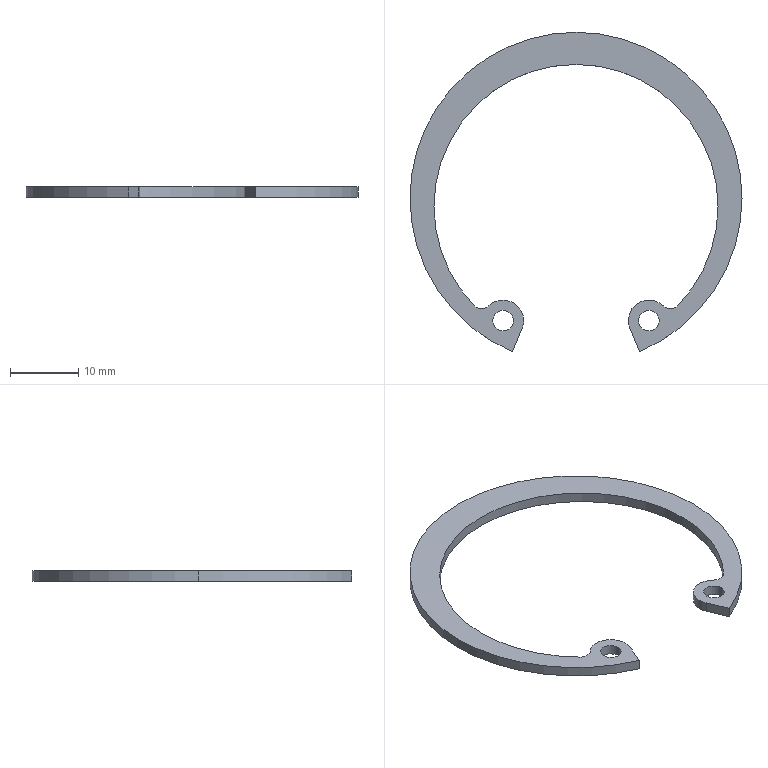Part | STEP file | circlips for holes--type a gb_GB_CONNECTING_PIECE_RING_RRH 45 | 1 solid | 19 faces | box 48.5 x 46.654 x 1.5 mm | volume 718.222 mm3 | cylinder 15 | plane 4 | commonest cylinder face diameters 3 x6 6 x3 41.5 x3 48.5 x3
STEP:
#1=CARTESIAN_POINT('',(24.25,0.,-1.5));
#2=VERTEX_POINT('',#1);
#3=CARTESIAN_POINT('',(-24.25,0.,-1.5));
#4=VERTEX_POINT('',#3);
#5=CARTESIAN_POINT('',(0.,0.,-1.5));
#6=DIRECTION('',(0.,0.,1.));
#7=DIRECTION('',(1.,0.,0.));
#8=AXIS2_PLACEMENT_3D('',#5,#6,#7);
#9=CIRCLE('',#8,24.25);
#10=EDGE_CURVE('',#2,#4,#9,.T.);
#11=ORIENTED_EDGE('',*,*,#10,.T.);
#12=CARTESIAN_POINT('',(-24.25,0.,0.));
#13=VERTEX_POINT('',#12);
#14=CARTESIAN_POINT('',(-24.25,0.,-1.5));
#15=DIRECTION('',(0.,0.,1.));
#16=VECTOR('',#15,1000.);
#17=LINE('',#14,#16);
#18=EDGE_CURVE('',#4,#13,#17,.T.);
#19=ORIENTED_EDGE('',*,*,#18,.T.);
#20=CARTESIAN_POINT('',(24.25,0.,0.));
#21=VERTEX_POINT('',#20);
#22=CARTESIAN_POINT('',(0.,0.,0.));
#23=DIRECTION('',(0.,0.,-1.));
#24=DIRECTION('',(1.,0.,0.));
#25=AXIS2_PLACEMENT_3D('',#22,#23,#24);
#26=CIRCLE('',#25,24.25);
#27=EDGE_CURVE('',#13,#21,#26,.T.);
#28=ORIENTED_EDGE('',*,*,#27,.T.);
#29=CARTESIAN_POINT('',(24.25,0.,-1.5));
#30=DIRECTION('',(0.,0.,1.));
#31=VECTOR('',#30,1000.);
#32=LINE('',#29,#31);
#33=EDGE_CURVE('',#2,#21,#32,.T.);
#34=ORIENTED_EDGE('',*,*,#33,.F.);
#35=EDGE_LOOP('',(#11,#19,#28,#34));
#36=FACE_OUTER_BOUND('',#35,.T.);
#37=CARTESIAN_POINT('',(0.,0.,-1.5));
#38=DIRECTION('',(0.,0.,1.));
#39=DIRECTION('',(1.,0.,0.));
#40=AXIS2_PLACEMENT_3D('',#37,#38,#39);
#41=CYLINDRICAL_SURFACE('',#40,24.25);
#42=ADVANCED_FACE('',(#36),#41,.T.);
#43=CARTESIAN_POINT('',(9.28,-22.404,-1.5));
#44=VERTEX_POINT('',#43);
#45=CARTESIAN_POINT('',(0.,0.,-1.5));
#46=DIRECTION('',(0.,0.,1.));
#47=DIRECTION('',(1.,0.,0.));
#48=AXIS2_PLACEMENT_3D('',#45,#46,#47);
#49=CIRCLE('',#48,24.25);
#50=EDGE_CURVE('',#44,#2,#49,.T.);
#51=ORIENTED_EDGE('',*,*,#50,.T.);
#52=ORIENTED_EDGE('',*,*,#33,.T.);
#53=CARTESIAN_POINT('',(9.28,-22.404,0.));
#54=VERTEX_POINT('',#53);
#55=CARTESIAN_POINT('',(0.,0.,0.));
#56=DIRECTION('',(0.,0.,-1.));
#57=DIRECTION('',(1.,0.,0.));
#58=AXIS2_PLACEMENT_3D('',#55,#56,#57);
#59=CIRCLE('',#58,24.25);
#60=EDGE_CURVE('',#21,#54,#59,.T.);
#61=ORIENTED_EDGE('',*,*,#60,.T.);
#62=CARTESIAN_POINT('',(9.28,-22.404,-1.5));
#63=DIRECTION('',(0.,0.,-1.));
#64=VECTOR('',#63,1000.);
#65=LINE('',#62,#64);
#66=EDGE_CURVE('',#54,#44,#65,.T.);
#67=ORIENTED_EDGE('',*,*,#66,.T.);
#68=EDGE_LOOP('',(#51,#52,#61,#67));
#69=FACE_OUTER_BOUND('',#68,.T.);
#70=CARTESIAN_POINT('',(0.,0.,-1.5));
#71=DIRECTION('',(0.,0.,1.));
#72=DIRECTION('',(1.,0.,0.));
#73=AXIS2_PLACEMENT_3D('',#70,#71,#72);
#74=CYLINDRICAL_SURFACE('',#73,24.25);
#75=ADVANCED_FACE('',(#69),#74,.T.);
#76=CARTESIAN_POINT('',(-14.857,-15.686,-1.5));
#77=VERTEX_POINT('',#76);
#78=CARTESIAN_POINT('',(-20.75,-1.2,-1.5));
#79=VERTEX_POINT('',#78);
#80=CARTESIAN_POINT('',(0.,-1.2,-1.5));
#81=DIRECTION('',(0.,0.,-1.));
#82=DIRECTION('',(1.,0.,0.));
#83=AXIS2_PLACEMENT_3D('',#80,#81,#82);
#84=CIRCLE('',#83,20.75);
#85=EDGE_CURVE('',#77,#79,#84,.T.);
#86=ORIENTED_EDGE('',*,*,#85,.T.);
#87=CARTESIAN_POINT('',(-20.75,-1.2,0.));
#88=VERTEX_POINT('',#87);
#89=CARTESIAN_POINT('',(-20.75,-1.2,-1.5));
#90=DIRECTION('',(0.,0.,1.));
#91=VECTOR('',#90,1000.);
#92=LINE('',#89,#91);
#93=EDGE_CURVE('',#79,#88,#92,.T.);
#94=ORIENTED_EDGE('',*,*,#93,.T.);
#95=CARTESIAN_POINT('',(-14.857,-15.686,0.));
#96=VERTEX_POINT('',#95);
#97=CARTESIAN_POINT('',(0.,-1.2,0.));
#98=DIRECTION('',(0.,0.,-1.));
#99=DIRECTION('',(1.,0.,0.));
#100=AXIS2_PLACEMENT_3D('',#97,#98,#99);
#101=CIRCLE('',#100,20.75);
#102=EDGE_CURVE('',#96,#88,#101,.T.);
#103=ORIENTED_EDGE('',*,*,#102,.F.);
#104=CARTESIAN_POINT('',(-14.857,-15.686,-1.5));
#105=DIRECTION('',(0.,0.,1.));
#106=VECTOR('',#105,1000.);
#107=LINE('',#104,#106);
#108=EDGE_CURVE('',#77,#96,#107,.T.);
#109=ORIENTED_EDGE('',*,*,#108,.F.);
#110=EDGE_LOOP('',(#86,#94,#103,#109));
#111=FACE_OUTER_BOUND('',#110,.T.);
#112=CARTESIAN_POINT('',(0.,-1.2,-1.5));
#113=DIRECTION('',(0.,0.,1.));
#114=DIRECTION('',(1.,0.,0.));
#115=AXIS2_PLACEMENT_3D('',#112,#113,#114);
#116=CYLINDRICAL_SURFACE('',#115,20.75);
#117=ADVANCED_FACE('',(#111),#116,.F.);
#118=ORIENTED_EDGE('',*,*,#93,.F.);
#119=CARTESIAN_POINT('',(20.75,-1.2,-1.5));
#120=VERTEX_POINT('',#119);
#121=CARTESIAN_POINT('',(0.,-1.2,-1.5));
#122=DIRECTION('',(0.,0.,-1.));
#123=DIRECTION('',(1.,0.,0.));
#124=AXIS2_PLACEMENT_3D('',#121,#122,#123);
#125=CIRCLE('',#124,20.75);
#126=EDGE_CURVE('',#79,#120,#125,.T.);
#127=ORIENTED_EDGE('',*,*,#126,.T.);
#128=CARTESIAN_POINT('',(20.75,-1.2,0.));
#129=VERTEX_POINT('',#128);
#130=CARTESIAN_POINT('',(20.75,-1.2,-1.5));
#131=DIRECTION('',(0.,0.,1.));
#132=VECTOR('',#131,1000.);
#133=LINE('',#130,#132);
#134=EDGE_CURVE('',#120,#129,#133,.T.);
#135=ORIENTED_EDGE('',*,*,#134,.T.);
#136=CARTESIAN_POINT('',(0.,-1.2,0.));
#137=DIRECTION('',(0.,0.,-1.));
#138=DIRECTION('',(1.,0.,0.));
#139=AXIS2_PLACEMENT_3D('',#136,#137,#138);
#140=CIRCLE('',#139,20.75);
#141=EDGE_CURVE('',#88,#129,#140,.T.);
#142=ORIENTED_EDGE('',*,*,#141,.F.);
#143=EDGE_LOOP('',(#118,#127,#135,#142));
#144=FACE_OUTER_BOUND('',#143,.T.);
#145=CARTESIAN_POINT('',(0.,-1.2,-1.5));
#146=DIRECTION('',(0.,0.,1.));
#147=DIRECTION('',(1.,0.,0.));
#148=AXIS2_PLACEMENT_3D('',#145,#146,#147);
#149=CYLINDRICAL_SURFACE('',#148,20.75);
#150=ADVANCED_FACE('',(#144),#149,.F.);
#151=CARTESIAN_POINT('',(-7.877,-19.016,-1.5));
#152=VERTEX_POINT('',#151);
#153=CARTESIAN_POINT('',(-7.648,-17.868,-1.5));
#154=VERTEX_POINT('',#153);
#155=CARTESIAN_POINT('',(-10.648,-17.868,-1.5));
#156=DIRECTION('',(0.,0.,1.));
#157=DIRECTION('',(1.,0.,0.));
#158=AXIS2_PLACEMENT_3D('',#155,#156,#157);
#159=CIRCLE('',#158,3.);
#160=EDGE_CURVE('',#152,#154,#159,.T.);
#161=ORIENTED_EDGE('',*,*,#160,.T.);
#162=CARTESIAN_POINT('',(-7.648,-17.868,0.));
#163=VERTEX_POINT('',#162);
#164=CARTESIAN_POINT('',(-7.648,-17.868,-1.5));
#165=DIRECTION('',(0.,0.,1.));
#166=VECTOR('',#165,1000.);
#167=LINE('',#164,#166);
#168=EDGE_CURVE('',#154,#163,#167,.T.);
#169=ORIENTED_EDGE('',*,*,#168,.T.);
#170=CARTESIAN_POINT('',(-7.877,-19.016,0.));
#171=VERTEX_POINT('',#170);
#172=CARTESIAN_POINT('',(-10.648,-17.868,0.));
#173=DIRECTION('',(0.,0.,-1.));
#174=DIRECTION('',(1.,0.,0.));
#175=AXIS2_PLACEMENT_3D('',#172,#173,#174);
#176=CIRCLE('',#175,3.);
#177=EDGE_CURVE('',#163,#171,#176,.T.);
#178=ORIENTED_EDGE('',*,*,#177,.T.);
#179=CARTESIAN_POINT('',(-7.877,-19.016,-1.5));
#180=DIRECTION('',(0.,0.,-1.));
#181=VECTOR('',#180,1000.);
#182=LINE('',#179,#181);
#183=EDGE_CURVE('',#171,#152,#182,.T.);
#184=ORIENTED_EDGE('',*,*,#183,.T.);
#185=EDGE_LOOP('',(#161,#169,#178,#184));
#186=FACE_OUTER_BOUND('',#185,.T.);
#187=CARTESIAN_POINT('',(-10.648,-17.868,-1.5));
#188=DIRECTION('',(0.,0.,1.));
#189=DIRECTION('',(1.,0.,0.));
#190=AXIS2_PLACEMENT_3D('',#187,#188,#189);
#191=CYLINDRICAL_SURFACE('',#190,3.);
#192=ADVANCED_FACE('',(#186),#191,.T.);
#193=CARTESIAN_POINT('',(12.148,-17.868,-1.5));
#194=VERTEX_POINT('',#193);
#195=CARTESIAN_POINT('',(9.148,-17.868,-1.5));
#196=VERTEX_POINT('',#195);
#197=CARTESIAN_POINT('',(10.648,-17.868,-1.5));
#198=DIRECTION('',(0.,0.,-1.));
#199=DIRECTION('',(1.,0.,0.));
#200=AXIS2_PLACEMENT_3D('',#197,#198,#199);
#201=CIRCLE('',#200,1.5);
#202=EDGE_CURVE('',#194,#196,#201,.T.);
#203=ORIENTED_EDGE('',*,*,#202,.T.);
#204=CARTESIAN_POINT('',(9.148,-17.868,0.));
#205=VERTEX_POINT('',#204);
#206=CARTESIAN_POINT('',(9.148,-17.868,-1.5));
#207=DIRECTION('',(0.,0.,1.));
#208=VECTOR('',#207,1000.);
#209=LINE('',#206,#208);
#210=EDGE_CURVE('',#196,#205,#209,.T.);
#211=ORIENTED_EDGE('',*,*,#210,.T.);
#212=CARTESIAN_POINT('',(12.148,-17.868,0.));
#213=VERTEX_POINT('',#212);
#214=CARTESIAN_POINT('',(10.648,-17.868,0.));
#215=DIRECTION('',(0.,0.,-1.));
#216=DIRECTION('',(1.,0.,0.));
#217=AXIS2_PLACEMENT_3D('',#214,#215,#216);
#218=CIRCLE('',#217,1.5);
#219=EDGE_CURVE('',#213,#205,#218,.T.);
#220=ORIENTED_EDGE('',*,*,#219,.F.);
#221=CARTESIAN_POINT('',(12.148,-17.868,-1.5));
#222=DIRECTION('',(0.,0.,1.));
#223=VECTOR('',#222,1000.);
#224=LINE('',#221,#223);
#225=EDGE_CURVE('',#194,#213,#224,.T.);
#226=ORIENTED_EDGE('',*,*,#225,.F.);
#227=EDGE_LOOP('',(#203,#211,#220,#226));
#228=FACE_OUTER_BOUND('',#227,.T.);
#229=CARTESIAN_POINT('',(10.648,-17.868,-1.5));
#230=DIRECTION('',(0.,0.,1.));
#231=DIRECTION('',(1.,0.,0.));
#232=AXIS2_PLACEMENT_3D('',#229,#230,#231);
#233=CYLINDRICAL_SURFACE('',#232,1.5);
#234=ADVANCED_FACE('',(#228),#233,.F.);
#235=CARTESIAN_POINT('',(-9.148,-17.868,-1.5));
#236=VERTEX_POINT('',#235);
#237=CARTESIAN_POINT('',(-12.148,-17.868,-1.5));
#238=VERTEX_POINT('',#237);
#239=CARTESIAN_POINT('',(-10.648,-17.868,-1.5));
#240=DIRECTION('',(0.,0.,-1.));
#241=DIRECTION('',(1.,0.,0.));
#242=AXIS2_PLACEMENT_3D('',#239,#240,#241);
#243=CIRCLE('',#242,1.5);
#244=EDGE_CURVE('',#236,#238,#243,.T.);
#245=ORIENTED_EDGE('',*,*,#244,.T.);
#246=CARTESIAN_POINT('',(-12.148,-17.868,0.));
#247=VERTEX_POINT('',#246);
#248=CARTESIAN_POINT('',(-12.148,-17.868,-1.5));
#249=DIRECTION('',(0.,0.,1.));
#250=VECTOR('',#249,1000.);
#251=LINE('',#248,#250);
#252=EDGE_CURVE('',#238,#247,#251,.T.);
#253=ORIENTED_EDGE('',*,*,#252,.T.);
#254=CARTESIAN_POINT('',(-9.148,-17.868,0.));
#255=VERTEX_POINT('',#254);
#256=CARTESIAN_POINT('',(-10.648,-17.868,0.));
#257=DIRECTION('',(0.,0.,-1.));
#258=DIRECTION('',(1.,0.,0.));
#259=AXIS2_PLACEMENT_3D('',#256,#257,#258);
#260=CIRCLE('',#259,1.5);
#261=EDGE_CURVE('',#255,#247,#260,.T.);
#262=ORIENTED_EDGE('',*,*,#261,.F.);
#263=CARTESIAN_POINT('',(-9.148,-17.868,-1.5));
#264=DIRECTION('',(0.,0.,1.));
#265=VECTOR('',#264,1000.);
#266=LINE('',#263,#265);
#267=EDGE_CURVE('',#236,#255,#266,.T.);
#268=ORIENTED_EDGE('',*,*,#267,.F.);
#269=EDGE_LOOP('',(#245,#253,#262,#268));
#270=FACE_OUTER_BOUND('',#269,.T.);
#271=CARTESIAN_POINT('',(-10.648,-17.868,-1.5));
#272=DIRECTION('',(0.,0.,1.));
#273=DIRECTION('',(1.,0.,0.));
#274=AXIS2_PLACEMENT_3D('',#271,#272,#273);
#275=CYLINDRICAL_SURFACE('',#274,1.5);
#276=ADVANCED_FACE('',(#270),#275,.F.);
#277=CARTESIAN_POINT('',(7.877,-19.016,-1.5));
#278=VERTEX_POINT('',#277);
#279=CARTESIAN_POINT('',(7.877,-19.016,-1.5));
#280=DIRECTION('',(0.3827,-0.9239,0.));
#281=VECTOR('',#280,1000.);
#282=LINE('',#279,#281);
#283=EDGE_CURVE('',#278,#44,#282,.T.);
#284=ORIENTED_EDGE('',*,*,#283,.F.);
#285=CARTESIAN_POINT('',(12.738,-15.715,-1.5));
#286=VERTEX_POINT('',#285);
#287=CARTESIAN_POINT('',(10.648,-17.868,-1.5));
#288=DIRECTION('',(0.,0.,1.));
#289=DIRECTION('',(1.,0.,0.));
#290=AXIS2_PLACEMENT_3D('',#287,#288,#289);
#291=CIRCLE('',#290,3.);
#292=EDGE_CURVE('',#286,#278,#291,.T.);
#293=ORIENTED_EDGE('',*,*,#292,.F.);
#294=CARTESIAN_POINT('',(14.857,-15.686,-1.5));
#295=VERTEX_POINT('',#294);
#296=CARTESIAN_POINT('',(13.783,-14.639,-1.5));
#297=DIRECTION('',(0.,0.,-1.));
#298=DIRECTION('',(1.,0.,0.));
#299=AXIS2_PLACEMENT_3D('',#296,#297,#298);
#300=CIRCLE('',#299,1.5);
#301=EDGE_CURVE('',#295,#286,#300,.T.);
#302=ORIENTED_EDGE('',*,*,#301,.F.);
#303=CARTESIAN_POINT('',(0.,-1.2,-1.5));
#304=DIRECTION('',(0.,0.,-1.));
#305=DIRECTION('',(1.,0.,0.));
#306=AXIS2_PLACEMENT_3D('',#303,#304,#305);
#307=CIRCLE('',#306,20.75);
#308=EDGE_CURVE('',#120,#295,#307,.T.);
#309=ORIENTED_EDGE('',*,*,#308,.F.);
#310=ORIENTED_EDGE('',*,*,#126,.F.);
#311=ORIENTED_EDGE('',*,*,#85,.F.);
#312=CARTESIAN_POINT('',(-12.738,-15.715,-1.5));
#313=VERTEX_POINT('',#312);
#314=CARTESIAN_POINT('',(-13.783,-14.639,-1.5));
#315=DIRECTION('',(0.,0.,-1.));
#316=DIRECTION('',(1.,0.,0.));
#317=AXIS2_PLACEMENT_3D('',#314,#315,#316);
#318=CIRCLE('',#317,1.5);
#319=EDGE_CURVE('',#313,#77,#318,.T.);
#320=ORIENTED_EDGE('',*,*,#319,.F.);
#321=CARTESIAN_POINT('',(-10.648,-17.868,-1.5));
#322=DIRECTION('',(0.,0.,1.));
#323=DIRECTION('',(1.,0.,0.));
#324=AXIS2_PLACEMENT_3D('',#321,#322,#323);
#325=CIRCLE('',#324,3.);
#326=EDGE_CURVE('',#154,#313,#325,.T.);
#327=ORIENTED_EDGE('',*,*,#326,.F.);
#328=ORIENTED_EDGE('',*,*,#160,.F.);
#329=CARTESIAN_POINT('',(-9.28,-22.404,-1.5));
#330=VERTEX_POINT('',#329);
#331=CARTESIAN_POINT('',(-9.28,-22.404,-1.5));
#332=DIRECTION('',(0.3827,0.9239,0.));
#333=VECTOR('',#332,1000.);
#334=LINE('',#331,#333);
#335=EDGE_CURVE('',#330,#152,#334,.T.);
#336=ORIENTED_EDGE('',*,*,#335,.F.);
#337=CARTESIAN_POINT('',(0.,0.,-1.5));
#338=DIRECTION('',(0.,0.,1.));
#339=DIRECTION('',(1.,0.,0.));
#340=AXIS2_PLACEMENT_3D('',#337,#338,#339);
#341=CIRCLE('',#340,24.25);
#342=EDGE_CURVE('',#4,#330,#341,.T.);
#343=ORIENTED_EDGE('',*,*,#342,.F.);
#344=ORIENTED_EDGE('',*,*,#10,.F.);
#345=ORIENTED_EDGE('',*,*,#50,.F.);
#346=EDGE_LOOP('',(#284,#293,#302,#309,#310,#311,#320,#327,#328,#336,#343,#344,#345));
#347=FACE_OUTER_BOUND('',#346,.T.);
#348=ORIENTED_EDGE('',*,*,#202,.F.);
#349=CARTESIAN_POINT('',(10.648,-17.868,-1.5));
#350=DIRECTION('',(0.,0.,-1.));
#351=DIRECTION('',(1.,0.,0.));
#352=AXIS2_PLACEMENT_3D('',#349,#350,#351);
#353=CIRCLE('',#352,1.5);
#354=EDGE_CURVE('',#196,#194,#353,.T.);
#355=ORIENTED_EDGE('',*,*,#354,.F.);
#356=EDGE_LOOP('',(#348,#355));
#357=FACE_BOUND('',#356,.T.);
#358=ORIENTED_EDGE('',*,*,#244,.F.);
#359=CARTESIAN_POINT('',(-10.648,-17.868,-1.5));
#360=DIRECTION('',(0.,0.,-1.));
#361=DIRECTION('',(1.,0.,0.));
#362=AXIS2_PLACEMENT_3D('',#359,#360,#361);
#363=CIRCLE('',#362,1.5);
#364=EDGE_CURVE('',#238,#236,#363,.T.);
#365=ORIENTED_EDGE('',*,*,#364,.F.);
#366=EDGE_LOOP('',(#358,#365));
#367=FACE_BOUND('',#366,.T.);
#368=CARTESIAN_POINT('',(0.,0.,-1.5));
#369=DIRECTION('',(0.,0.,1.));
#370=DIRECTION('',(1.,0.,0.));
#371=AXIS2_PLACEMENT_3D('',#368,#369,#370);
#372=PLANE('',#371);
#373=ADVANCED_FACE('',(#347,#357,#367),#372,.F.);
#374=ORIENTED_EDGE('',*,*,#18,.F.);
#375=ORIENTED_EDGE('',*,*,#342,.T.);
#376=CARTESIAN_POINT('',(-9.28,-22.404,0.));
#377=VERTEX_POINT('',#376);
#378=CARTESIAN_POINT('',(-9.28,-22.404,-1.5));
#379=DIRECTION('',(0.,0.,-1.));
#380=VECTOR('',#379,1000.);
#381=LINE('',#378,#380);
#382=EDGE_CURVE('',#377,#330,#381,.T.);
#383=ORIENTED_EDGE('',*,*,#382,.F.);
#384=CARTESIAN_POINT('',(0.,0.,0.));
#385=DIRECTION('',(0.,0.,-1.));
#386=DIRECTION('',(1.,0.,0.));
#387=AXIS2_PLACEMENT_3D('',#384,#385,#386);
#388=CIRCLE('',#387,24.25);
#389=EDGE_CURVE('',#377,#13,#388,.T.);
#390=ORIENTED_EDGE('',*,*,#389,.T.);
#391=EDGE_LOOP('',(#374,#375,#383,#390));
#392=FACE_OUTER_BOUND('',#391,.T.);
#393=CARTESIAN_POINT('',(0.,0.,-1.5));
#394=DIRECTION('',(0.,0.,1.));
#395=DIRECTION('',(1.,0.,0.));
#396=AXIS2_PLACEMENT_3D('',#393,#394,#395);
#397=CYLINDRICAL_SURFACE('',#396,24.25);
#398=ADVANCED_FACE('',(#392),#397,.T.);
#399=ORIENTED_EDGE('',*,*,#283,.T.);
#400=ORIENTED_EDGE('',*,*,#66,.F.);
#401=CARTESIAN_POINT('',(7.877,-19.016,0.));
#402=VERTEX_POINT('',#401);
#403=CARTESIAN_POINT('',(7.877,-19.016,0.));
#404=DIRECTION('',(-0.3827,0.9239,0.));
#405=VECTOR('',#404,1000.);
#406=LINE('',#403,#405);
#407=EDGE_CURVE('',#54,#402,#406,.T.);
#408=ORIENTED_EDGE('',*,*,#407,.T.);
#409=CARTESIAN_POINT('',(7.877,-19.016,-1.5));
#410=DIRECTION('',(0.,0.,-1.));
#411=VECTOR('',#410,1000.);
#412=LINE('',#409,#411);
#413=EDGE_CURVE('',#402,#278,#412,.T.);
#414=ORIENTED_EDGE('',*,*,#413,.T.);
#415=EDGE_LOOP('',(#399,#400,#408,#414));
#416=FACE_OUTER_BOUND('',#415,.T.);
#417=CARTESIAN_POINT('',(7.877,-19.016,-1.5));
#418=DIRECTION('',(-0.9239,-0.3827,0.));
#419=DIRECTION('',(0.3827,-0.9239,0.));
#420=AXIS2_PLACEMENT_3D('',#417,#418,#419);
#421=PLANE('',#420);
#422=ADVANCED_FACE('',(#416),#421,.T.);
#423=ORIENTED_EDGE('',*,*,#292,.T.);
#424=ORIENTED_EDGE('',*,*,#413,.F.);
#425=CARTESIAN_POINT('',(12.738,-15.715,0.));
#426=VERTEX_POINT('',#425);
#427=CARTESIAN_POINT('',(10.648,-17.868,0.));
#428=DIRECTION('',(0.,0.,-1.));
#429=DIRECTION('',(1.,0.,0.));
#430=AXIS2_PLACEMENT_3D('',#427,#428,#429);
#431=CIRCLE('',#430,3.);
#432=EDGE_CURVE('',#402,#426,#431,.T.);
#433=ORIENTED_EDGE('',*,*,#432,.T.);
#434=CARTESIAN_POINT('',(12.738,-15.715,-1.5));
#435=DIRECTION('',(0.,0.,-1.));
#436=VECTOR('',#435,1000.);
#437=LINE('',#434,#436);
#438=EDGE_CURVE('',#426,#286,#437,.T.);
#439=ORIENTED_EDGE('',*,*,#438,.T.);
#440=EDGE_LOOP('',(#423,#424,#433,#439));
#441=FACE_OUTER_BOUND('',#440,.T.);
#442=CARTESIAN_POINT('',(10.648,-17.868,-1.5));
#443=DIRECTION('',(0.,0.,1.));
#444=DIRECTION('',(1.,0.,0.));
#445=AXIS2_PLACEMENT_3D('',#442,#443,#444);
#446=CYLINDRICAL_SURFACE('',#445,3.);
#447=ADVANCED_FACE('',(#441),#446,.T.);
#448=CARTESIAN_POINT('',(14.857,-15.686,0.));
#449=VERTEX_POINT('',#448);
#450=CARTESIAN_POINT('',(14.857,-15.686,-1.5));
#451=DIRECTION('',(0.,0.,1.));
#452=VECTOR('',#451,1000.);
#453=LINE('',#450,#452);
#454=EDGE_CURVE('',#295,#449,#453,.T.);
#455=ORIENTED_EDGE('',*,*,#454,.F.);
#456=ORIENTED_EDGE('',*,*,#301,.T.);
#457=ORIENTED_EDGE('',*,*,#438,.F.);
#458=CARTESIAN_POINT('',(13.783,-14.639,0.));
#459=DIRECTION('',(0.,0.,-1.));
#460=DIRECTION('',(1.,0.,0.));
#461=AXIS2_PLACEMENT_3D('',#458,#459,#460);
#462=CIRCLE('',#461,1.5);
#463=EDGE_CURVE('',#449,#426,#462,.T.);
#464=ORIENTED_EDGE('',*,*,#463,.F.);
#465=EDGE_LOOP('',(#455,#456,#457,#464));
#466=FACE_OUTER_BOUND('',#465,.T.);
#467=CARTESIAN_POINT('',(13.783,-14.639,-1.5));
#468=DIRECTION('',(0.,0.,1.));
#469=DIRECTION('',(1.,0.,0.));
#470=AXIS2_PLACEMENT_3D('',#467,#468,#469);
#471=CYLINDRICAL_SURFACE('',#470,1.5);
#472=ADVANCED_FACE('',(#466),#471,.F.);
#473=ORIENTED_EDGE('',*,*,#134,.F.);
#474=ORIENTED_EDGE('',*,*,#308,.T.);
#475=ORIENTED_EDGE('',*,*,#454,.T.);
#476=CARTESIAN_POINT('',(0.,-1.2,0.));
#477=DIRECTION('',(0.,0.,-1.));
#478=DIRECTION('',(1.,0.,0.));
#479=AXIS2_PLACEMENT_3D('',#476,#477,#478);
#480=CIRCLE('',#479,20.75);
#481=EDGE_CURVE('',#129,#449,#480,.T.);
#482=ORIENTED_EDGE('',*,*,#481,.F.);
#483=EDGE_LOOP('',(#473,#474,#475,#482));
#484=FACE_OUTER_BOUND('',#483,.T.);
#485=CARTESIAN_POINT('',(0.,-1.2,-1.5));
#486=DIRECTION('',(0.,0.,1.));
#487=DIRECTION('',(1.,0.,0.));
#488=AXIS2_PLACEMENT_3D('',#485,#486,#487);
#489=CYLINDRICAL_SURFACE('',#488,20.75);
#490=ADVANCED_FACE('',(#484),#489,.F.);
#491=CARTESIAN_POINT('',(-12.738,-15.715,0.));
#492=VERTEX_POINT('',#491);
#493=CARTESIAN_POINT('',(-12.738,-15.715,-1.5));
#494=DIRECTION('',(0.,0.,1.));
#495=VECTOR('',#494,1000.);
#496=LINE('',#493,#495);
#497=EDGE_CURVE('',#313,#492,#496,.T.);
#498=ORIENTED_EDGE('',*,*,#497,.F.);
#499=ORIENTED_EDGE('',*,*,#319,.T.);
#500=ORIENTED_EDGE('',*,*,#108,.T.);
#501=CARTESIAN_POINT('',(-13.783,-14.639,0.));
#502=DIRECTION('',(0.,0.,-1.));
#503=DIRECTION('',(1.,0.,0.));
#504=AXIS2_PLACEMENT_3D('',#501,#502,#503);
#505=CIRCLE('',#504,1.5);
#506=EDGE_CURVE('',#492,#96,#505,.T.);
#507=ORIENTED_EDGE('',*,*,#506,.F.);
#508=EDGE_LOOP('',(#498,#499,#500,#507));
#509=FACE_OUTER_BOUND('',#508,.T.);
#510=CARTESIAN_POINT('',(-13.783,-14.639,-1.5));
#511=DIRECTION('',(0.,0.,1.));
#512=DIRECTION('',(1.,0.,0.));
#513=AXIS2_PLACEMENT_3D('',#510,#511,#512);
#514=CYLINDRICAL_SURFACE('',#513,1.5);
#515=ADVANCED_FACE('',(#509),#514,.F.);
#516=ORIENTED_EDGE('',*,*,#168,.F.);
#517=ORIENTED_EDGE('',*,*,#326,.T.);
#518=ORIENTED_EDGE('',*,*,#497,.T.);
#519=CARTESIAN_POINT('',(-10.648,-17.868,0.));
#520=DIRECTION('',(0.,0.,-1.));
#521=DIRECTION('',(1.,0.,0.));
#522=AXIS2_PLACEMENT_3D('',#519,#520,#521);
#523=CIRCLE('',#522,3.);
#524=EDGE_CURVE('',#492,#163,#523,.T.);
#525=ORIENTED_EDGE('',*,*,#524,.T.);
#526=EDGE_LOOP('',(#516,#517,#518,#525));
#527=FACE_OUTER_BOUND('',#526,.T.);
#528=CARTESIAN_POINT('',(-10.648,-17.868,-1.5));
#529=DIRECTION('',(0.,0.,1.));
#530=DIRECTION('',(1.,0.,0.));
#531=AXIS2_PLACEMENT_3D('',#528,#529,#530);
#532=CYLINDRICAL_SURFACE('',#531,3.);
#533=ADVANCED_FACE('',(#527),#532,.T.);
#534=ORIENTED_EDGE('',*,*,#335,.T.);
#535=ORIENTED_EDGE('',*,*,#183,.F.);
#536=CARTESIAN_POINT('',(-7.877,-19.016,0.));
#537=DIRECTION('',(-0.3827,-0.9239,0.));
#538=VECTOR('',#537,1000.);
#539=LINE('',#536,#538);
#540=EDGE_CURVE('',#171,#377,#539,.T.);
#541=ORIENTED_EDGE('',*,*,#540,.T.);
#542=ORIENTED_EDGE('',*,*,#382,.T.);
#543=EDGE_LOOP('',(#534,#535,#541,#542));
#544=FACE_OUTER_BOUND('',#543,.T.);
#545=CARTESIAN_POINT('',(-7.877,-19.016,-1.5));
#546=DIRECTION('',(0.9239,-0.3827,0.));
#547=DIRECTION('',(0.3827,0.9239,0.));
#548=AXIS2_PLACEMENT_3D('',#545,#546,#547);
#549=PLANE('',#548);
#550=ADVANCED_FACE('',(#544),#549,.T.);
#551=ORIENTED_EDGE('',*,*,#210,.F.);
#552=ORIENTED_EDGE('',*,*,#354,.T.);
#553=ORIENTED_EDGE('',*,*,#225,.T.);
#554=CARTESIAN_POINT('',(10.648,-17.868,0.));
#555=DIRECTION('',(0.,0.,-1.));
#556=DIRECTION('',(1.,0.,0.));
#557=AXIS2_PLACEMENT_3D('',#554,#555,#556);
#558=CIRCLE('',#557,1.5);
#559=EDGE_CURVE('',#205,#213,#558,.T.);
#560=ORIENTED_EDGE('',*,*,#559,.F.);
#561=EDGE_LOOP('',(#551,#552,#553,#560));
#562=FACE_OUTER_BOUND('',#561,.T.);
#563=CARTESIAN_POINT('',(10.648,-17.868,-1.5));
#564=DIRECTION('',(0.,0.,1.));
#565=DIRECTION('',(1.,0.,0.));
#566=AXIS2_PLACEMENT_3D('',#563,#564,#565);
#567=CYLINDRICAL_SURFACE('',#566,1.5);
#568=ADVANCED_FACE('',(#562),#567,.F.);
#569=ORIENTED_EDGE('',*,*,#252,.F.);
#570=ORIENTED_EDGE('',*,*,#364,.T.);
#571=ORIENTED_EDGE('',*,*,#267,.T.);
#572=CARTESIAN_POINT('',(-10.648,-17.868,0.));
#573=DIRECTION('',(0.,0.,-1.));
#574=DIRECTION('',(1.,0.,0.));
#575=AXIS2_PLACEMENT_3D('',#572,#573,#574);
#576=CIRCLE('',#575,1.5);
#577=EDGE_CURVE('',#247,#255,#576,.T.);
#578=ORIENTED_EDGE('',*,*,#577,.F.);
#579=EDGE_LOOP('',(#569,#570,#571,#578));
#580=FACE_OUTER_BOUND('',#579,.T.);
#581=CARTESIAN_POINT('',(-10.648,-17.868,-1.5));
#582=DIRECTION('',(0.,0.,1.));
#583=DIRECTION('',(1.,0.,0.));
#584=AXIS2_PLACEMENT_3D('',#581,#582,#583);
#585=CYLINDRICAL_SURFACE('',#584,1.5);
#586=ADVANCED_FACE('',(#580),#585,.F.);
#587=ORIENTED_EDGE('',*,*,#432,.F.);
#588=ORIENTED_EDGE('',*,*,#407,.F.);
#589=ORIENTED_EDGE('',*,*,#60,.F.);
#590=ORIENTED_EDGE('',*,*,#27,.F.);
#591=ORIENTED_EDGE('',*,*,#389,.F.);
#592=ORIENTED_EDGE('',*,*,#540,.F.);
#593=ORIENTED_EDGE('',*,*,#177,.F.);
#594=ORIENTED_EDGE('',*,*,#524,.F.);
#595=ORIENTED_EDGE('',*,*,#506,.T.);
#596=ORIENTED_EDGE('',*,*,#102,.T.);
#597=ORIENTED_EDGE('',*,*,#141,.T.);
#598=ORIENTED_EDGE('',*,*,#481,.T.);
#599=ORIENTED_EDGE('',*,*,#463,.T.);
#600=EDGE_LOOP('',(#587,#588,#589,#590,#591,#592,#593,#594,#595,#596,#597,#598,#599));
#601=FACE_OUTER_BOUND('',#600,.T.);
#602=ORIENTED_EDGE('',*,*,#219,.T.);
#603=ORIENTED_EDGE('',*,*,#559,.T.);
#604=EDGE_LOOP('',(#602,#603));
#605=FACE_BOUND('',#604,.T.);
#606=ORIENTED_EDGE('',*,*,#261,.T.);
#607=ORIENTED_EDGE('',*,*,#577,.T.);
#608=EDGE_LOOP('',(#606,#607));
#609=FACE_BOUND('',#608,.T.);
#610=CARTESIAN_POINT('',(0.,0.,0.));
#611=DIRECTION('',(0.,0.,1.));
#612=DIRECTION('',(1.,0.,0.));
#613=AXIS2_PLACEMENT_3D('',#610,#611,#612);
#614=PLANE('',#613);
#615=ADVANCED_FACE('',(#601,#605,#609),#614,.T.);
#616=CLOSED_SHELL('',(#42,#75,#117,#150,#192,#234,#276,#373,#398,#422,#447,#472,#490,#515,#533,#550,#568,#586,#615));
#617=MANIFOLD_SOLID_BREP('',#616);
#618=CARTESIAN_POINT('',(0.,0.,0.));
#619=DIRECTION('',(0.,0.,1.));
#620=DIRECTION('',(1.,0.,0.));
#621=AXIS2_PLACEMENT_3D('',#618,#619,#620);
#622=(LENGTH_UNIT()NAMED_UNIT(*)SI_UNIT(.MILLI.,.METRE.));
#623=UNCERTAINTY_MEASURE_WITH_UNIT(LENGTH_MEASURE(0.00001),#622,'','');
#624=(NAMED_UNIT(*)PLANE_ANGLE_UNIT()SI_UNIT($,.RADIAN.));
#625=(NAMED_UNIT(*)SI_UNIT($,.STERADIAN.)SOLID_ANGLE_UNIT());
#626=(GEOMETRIC_REPRESENTATION_CONTEXT(3)GLOBAL_UNCERTAINTY_ASSIGNED_CONTEXT((#623))GLOBAL_UNIT_ASSIGNED_CONTEXT((#622,#624,#625))REPRESENTATION_CONTEXT('',''));
#627=ADVANCED_BREP_SHAPE_REPRESENTATION('',(#617,#621),#626);